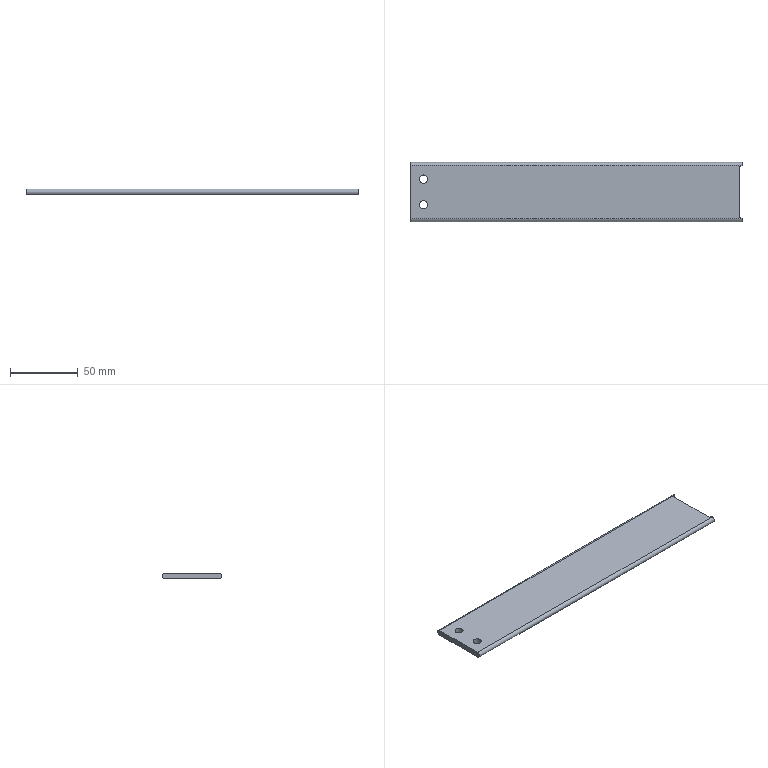Part | STEP file | Tube feed_id910_x_t | 1 solid | 12 faces | box 244.5 x 43.6 x 4.2 mm | volume 43290 mm3 | plane 8 | cylinder 4 | commonest cylinder face diameters 4.2 x2 6 x2
STEP:
#1=CARTESIAN_POINT('',(0.,0.,0.));
#2=DIRECTION('',(0.,0.,1.));
#3=DIRECTION('',(1.,0.,0.));
#4=AXIS2_PLACEMENT_3D('',#1,#2,#3);
#5=CARTESIAN_POINT('',(-309.5,-9.325,-1.3));
#6=VERTEX_POINT('',#5);
#7=CARTESIAN_POINT('',(-309.5,-9.664,-1.3));
#8=VERTEX_POINT('',#7);
#9=CARTESIAN_POINT('',(-309.5,29.736,-1.3));
#10=DIRECTION('',(0.,-1.,0.));
#11=VECTOR('',#10,1.);
#12=LINE('',#9,#11);
#13=CARTESIAN_POINT('',(-554.,29.736,-1.3));
#14=DIRECTION('',(0.,0.,1.));
#15=DIRECTION('',(0.,-1.,0.));
#16=AXIS2_PLACEMENT_3D('',#13,#14,#15);
#17=PLANE('',#16);
#18=CARTESIAN_POINT('',(0.,244.5));
#19=DIRECTION('',(1.,0.));
#20=VECTOR('',#19,1.);
#21=LINE('',#18,#20);
#22=(GEOMETRIC_REPRESENTATION_CONTEXT(2)PARAMETRIC_REPRESENTATION_CONTEXT()REPRESENTATION_CONTEXT('',''));
#23=DEFINITIONAL_REPRESENTATION('',(#21),#22);
#24=PCURVE('',#17,#23);
#25=CARTESIAN_POINT('',(-309.5,29.736,-3.15));
#26=DIRECTION('',(1.,0.,0.));
#27=DIRECTION('',(0.,0.,-1.));
#28=AXIS2_PLACEMENT_3D('',#25,#26,#27);
#29=PLANE('',#28);
#30=CARTESIAN_POINT('',(-1.85,0.));
#31=DIRECTION('',(0.,-1.));
#32=VECTOR('',#31,1.);
#33=LINE('',#30,#32);
#34=(GEOMETRIC_REPRESENTATION_CONTEXT(2)PARAMETRIC_REPRESENTATION_CONTEXT()REPRESENTATION_CONTEXT('',''));
#35=DEFINITIONAL_REPRESENTATION('',(#33),#34);
#36=PCURVE('',#29,#35);
#37=SURFACE_CURVE('',#12,(#24,#36),.PCURVE_S1.);
#38=EDGE_CURVE('',#6,#8,#37,.T.);
#39=ORIENTED_EDGE('',*,*,#38,.F.);
#40=CARTESIAN_POINT('',(-311.5,-8.629,-1.3));
#41=VERTEX_POINT('',#40);
#42=CARTESIAN_POINT('',(-539.725,70.769,-1.3));
#43=DIRECTION('',(-0.9445,0.3286,0.));
#44=VECTOR('',#43,1.);
#45=LINE('',#42,#44);
#46=CARTESIAN_POINT('',(-41.033,14.275));
#47=DIRECTION('',(-0.3286,-0.9445));
#48=VECTOR('',#47,1.);
#49=LINE('',#46,#48);
#50=(GEOMETRIC_REPRESENTATION_CONTEXT(2)PARAMETRIC_REPRESENTATION_CONTEXT()REPRESENTATION_CONTEXT('',''));
#51=DEFINITIONAL_REPRESENTATION('',(#49),#50);
#52=PCURVE('',#17,#51);
#53=CARTESIAN_POINT('',(-311.5,-8.629,48.7));
#54=DIRECTION('',(0.3286,0.9445,0.));
#55=DIRECTION('',(-0.9445,0.3286,0.));
#56=AXIS2_PLACEMENT_3D('',#53,#54,#55);
#57=PLANE('',#56);
#58=CARTESIAN_POINT('',(241.642,-50.));
#59=DIRECTION('',(1.,0.));
#60=VECTOR('',#59,1.);
#61=LINE('',#58,#60);
#62=(GEOMETRIC_REPRESENTATION_CONTEXT(2)PARAMETRIC_REPRESENTATION_CONTEXT()REPRESENTATION_CONTEXT('',''));
#63=DEFINITIONAL_REPRESENTATION('',(#61),#62);
#64=PCURVE('',#57,#63);
#65=SURFACE_CURVE('',#45,(#52,#64),.PCURVE_S1.);
#66=EDGE_CURVE('',#6,#41,#65,.T.);
#67=ORIENTED_EDGE('',*,*,#66,.T.);
#68=CARTESIAN_POINT('',(-311.5,28.701,-1.3));
#69=VERTEX_POINT('',#68);
#70=CARTESIAN_POINT('',(-311.5,29.736,-1.3));
#71=DIRECTION('',(0.,1.,0.));
#72=VECTOR('',#71,1.);
#73=LINE('',#70,#72);
#74=CARTESIAN_POINT('',(0.,242.5));
#75=DIRECTION('',(-1.,0.));
#76=VECTOR('',#75,1.);
#77=LINE('',#74,#76);
#78=(GEOMETRIC_REPRESENTATION_CONTEXT(2)PARAMETRIC_REPRESENTATION_CONTEXT()REPRESENTATION_CONTEXT('',''));
#79=DEFINITIONAL_REPRESENTATION('',(#77),#78);
#80=PCURVE('',#17,#79);
#81=CARTESIAN_POINT('',(-311.5,28.701,48.7));
#82=DIRECTION('',(1.,0.,0.));
#83=DIRECTION('',(0.,0.,-1.));
#84=AXIS2_PLACEMENT_3D('',#81,#82,#83);
#85=PLANE('',#84);
#86=CARTESIAN_POINT('',(50.,1.035));
#87=DIRECTION('',(0.,1.));
#88=VECTOR('',#87,1.);
#89=LINE('',#86,#88);
#90=(GEOMETRIC_REPRESENTATION_CONTEXT(2)PARAMETRIC_REPRESENTATION_CONTEXT()REPRESENTATION_CONTEXT('',''));
#91=DEFINITIONAL_REPRESENTATION('',(#89),#90);
#92=PCURVE('',#85,#91);
#93=SURFACE_CURVE('',#73,(#80,#92),.PCURVE_S1.);
#94=EDGE_CURVE('',#41,#69,#93,.T.);
#95=ORIENTED_EDGE('',*,*,#94,.T.);
#96=CARTESIAN_POINT('',(-309.5,29.396,-1.3));
#97=VERTEX_POINT('',#96);
#98=CARTESIAN_POINT('',(-527.498,-46.444,-1.3));
#99=DIRECTION('',(0.9445,0.3286,0.));
#100=VECTOR('',#99,1.);
#101=LINE('',#98,#100);
#102=CARTESIAN_POINT('',(76.179,26.502));
#103=DIRECTION('',(-0.3286,0.9445));
#104=VECTOR('',#103,1.);
#105=LINE('',#102,#104);
#106=(GEOMETRIC_REPRESENTATION_CONTEXT(2)PARAMETRIC_REPRESENTATION_CONTEXT()REPRESENTATION_CONTEXT('',''));
#107=DEFINITIONAL_REPRESENTATION('',(#105),#106);
#108=PCURVE('',#17,#107);
#109=CARTESIAN_POINT('',(-302.,32.005,48.7));
#110=DIRECTION('',(0.3286,-0.9445,0.));
#111=DIRECTION('',(0.9445,0.3286,0.));
#112=AXIS2_PLACEMENT_3D('',#109,#110,#111);
#113=PLANE('',#112);
#114=CARTESIAN_POINT('',(-238.754,-50.));
#115=DIRECTION('',(1.,0.));
#116=VECTOR('',#115,1.);
#117=LINE('',#114,#116);
#118=(GEOMETRIC_REPRESENTATION_CONTEXT(2)PARAMETRIC_REPRESENTATION_CONTEXT()REPRESENTATION_CONTEXT('',''));
#119=DEFINITIONAL_REPRESENTATION('',(#117),#118);
#120=PCURVE('',#113,#119);
#121=SURFACE_CURVE('',#101,(#108,#120),.PCURVE_S1.);
#122=EDGE_CURVE('',#69,#97,#121,.T.);
#123=ORIENTED_EDGE('',*,*,#122,.T.);
#124=CARTESIAN_POINT('',(-309.5,29.736,-1.3));
#125=VERTEX_POINT('',#124);
#126=CARTESIAN_POINT('',(-309.5,29.736,-1.3));
#127=DIRECTION('',(0.,-1.,0.));
#128=VECTOR('',#127,1.);
#129=LINE('',#126,#128);
#130=CARTESIAN_POINT('',(0.,244.5));
#131=DIRECTION('',(1.,0.));
#132=VECTOR('',#131,1.);
#133=LINE('',#130,#132);
#134=(GEOMETRIC_REPRESENTATION_CONTEXT(2)PARAMETRIC_REPRESENTATION_CONTEXT()REPRESENTATION_CONTEXT('',''));
#135=DEFINITIONAL_REPRESENTATION('',(#133),#134);
#136=PCURVE('',#17,#135);
#137=CARTESIAN_POINT('',(-309.5,29.736,-3.15));
#138=DIRECTION('',(1.,0.,0.));
#139=DIRECTION('',(0.,0.,-1.));
#140=AXIS2_PLACEMENT_3D('',#137,#138,#139);
#141=PLANE('',#140);
#142=CARTESIAN_POINT('',(-1.85,0.));
#143=DIRECTION('',(0.,-1.));
#144=VECTOR('',#143,1.);
#145=LINE('',#142,#144);
#146=(GEOMETRIC_REPRESENTATION_CONTEXT(2)PARAMETRIC_REPRESENTATION_CONTEXT()REPRESENTATION_CONTEXT('',''));
#147=DEFINITIONAL_REPRESENTATION('',(#145),#146);
#148=PCURVE('',#141,#147);
#149=SURFACE_CURVE('',#129,(#136,#148),.PCURVE_S1.);
#150=EDGE_CURVE('',#125,#97,#149,.T.);
#151=ORIENTED_EDGE('',*,*,#150,.F.);
#152=CARTESIAN_POINT('',(-554.,29.736,-1.3));
#153=VERTEX_POINT('',#152);
#154=CARTESIAN_POINT('',(-401.5,29.736,-1.3));
#155=DIRECTION('',(1.,0.,0.));
#156=VECTOR('',#155,1.);
#157=LINE('',#154,#156);
#158=CARTESIAN_POINT('',(0.,152.5));
#159=DIRECTION('',(0.,1.));
#160=VECTOR('',#159,1.);
#161=LINE('',#158,#160);
#162=(GEOMETRIC_REPRESENTATION_CONTEXT(2)PARAMETRIC_REPRESENTATION_CONTEXT()REPRESENTATION_CONTEXT('',''));
#163=DEFINITIONAL_REPRESENTATION('',(#161),#162);
#164=PCURVE('',#17,#163);
#165=CARTESIAN_POINT('',(-554.,29.736,-3.4));
#166=DIRECTION('',(1.,0.,0.));
#167=DIRECTION('',(0.,0.,-1.));
#168=AXIS2_PLACEMENT_3D('',#165,#166,#167);
#169=CYLINDRICAL_SURFACE('',#168,2.1);
#170=CARTESIAN_POINT('',(3.142,152.5));
#171=DIRECTION('',(0.,1.));
#172=VECTOR('',#171,1.);
#173=LINE('',#170,#172);
#174=(GEOMETRIC_REPRESENTATION_CONTEXT(2)PARAMETRIC_REPRESENTATION_CONTEXT()REPRESENTATION_CONTEXT('',''));
#175=DEFINITIONAL_REPRESENTATION('',(#173),#174);
#176=PCURVE('',#169,#175);
#177=SURFACE_CURVE('',#157,(#164,#176),.PCURVE_S1.);
#178=EDGE_CURVE('',#153,#125,#177,.T.);
#179=ORIENTED_EDGE('',*,*,#178,.F.);
#180=CARTESIAN_POINT('',(-554.,-9.664,-1.3));
#181=VERTEX_POINT('',#180);
#182=CARTESIAN_POINT('',(-554.,29.736,-1.3));
#183=DIRECTION('',(0.,-1.,0.));
#184=VECTOR('',#183,1.);
#185=LINE('',#182,#184);
#186=CARTESIAN_POINT('',(0.,0.));
#187=DIRECTION('',(1.,0.));
#188=VECTOR('',#187,1.);
#189=LINE('',#186,#188);
#190=(GEOMETRIC_REPRESENTATION_CONTEXT(2)PARAMETRIC_REPRESENTATION_CONTEXT()REPRESENTATION_CONTEXT('',''));
#191=DEFINITIONAL_REPRESENTATION('',(#189),#190);
#192=PCURVE('',#17,#191);
#193=CARTESIAN_POINT('',(-554.,29.736,-3.15));
#194=DIRECTION('',(1.,0.,0.));
#195=DIRECTION('',(0.,0.,-1.));
#196=AXIS2_PLACEMENT_3D('',#193,#194,#195);
#197=PLANE('',#196);
#198=CARTESIAN_POINT('',(-1.85,0.));
#199=DIRECTION('',(0.,-1.));
#200=VECTOR('',#199,1.);
#201=LINE('',#198,#200);
#202=(GEOMETRIC_REPRESENTATION_CONTEXT(2)PARAMETRIC_REPRESENTATION_CONTEXT()REPRESENTATION_CONTEXT('',''));
#203=DEFINITIONAL_REPRESENTATION('',(#201),#202);
#204=PCURVE('',#197,#203);
#205=SURFACE_CURVE('',#185,(#192,#204),.PCURVE_S1.);
#206=EDGE_CURVE('',#153,#181,#205,.T.);
#207=ORIENTED_EDGE('',*,*,#206,.T.);
#208=CARTESIAN_POINT('',(-401.5,-9.664,-1.3));
#209=DIRECTION('',(1.,0.,0.));
#210=VECTOR('',#209,1.);
#211=LINE('',#208,#210);
#212=CARTESIAN_POINT('',(39.4,152.5));
#213=DIRECTION('',(0.,1.));
#214=VECTOR('',#213,1.);
#215=LINE('',#212,#214);
#216=(GEOMETRIC_REPRESENTATION_CONTEXT(2)PARAMETRIC_REPRESENTATION_CONTEXT()REPRESENTATION_CONTEXT('',''));
#217=DEFINITIONAL_REPRESENTATION('',(#215),#216);
#218=PCURVE('',#17,#217);
#219=CARTESIAN_POINT('',(-554.,-9.664,-3.4));
#220=DIRECTION('',(1.,0.,0.));
#221=DIRECTION('',(0.,0.,-1.));
#222=AXIS2_PLACEMENT_3D('',#219,#220,#221);
#223=CYLINDRICAL_SURFACE('',#222,2.1);
#224=CARTESIAN_POINT('',(3.142,152.5));
#225=DIRECTION('',(0.,1.));
#226=VECTOR('',#225,1.);
#227=LINE('',#224,#226);
#228=(GEOMETRIC_REPRESENTATION_CONTEXT(2)PARAMETRIC_REPRESENTATION_CONTEXT()REPRESENTATION_CONTEXT('',''));
#229=DEFINITIONAL_REPRESENTATION('',(#227),#228);
#230=PCURVE('',#223,#229);
#231=SURFACE_CURVE('',#211,(#218,#230),.PCURVE_S1.);
#232=EDGE_CURVE('',#181,#8,#231,.T.);
#233=ORIENTED_EDGE('',*,*,#232,.T.);
#234=EDGE_LOOP('',(#39,#67,#95,#123,#151,#179,#207,#233));
#235=FACE_BOUND('',#234,.T.);
#236=CARTESIAN_POINT('',(-544.,16.556,-1.3));
#237=VERTEX_POINT('',#236);
#238=CARTESIAN_POINT('',(-544.,22.556,-1.3));
#239=VERTEX_POINT('',#238);
#240=CARTESIAN_POINT('',(-544.,19.556,-1.3));
#241=DIRECTION('',(0.,0.,1.));
#242=DIRECTION('',(0.,-1.,0.));
#243=AXIS2_PLACEMENT_3D('',#240,#241,#242);
#244=CIRCLE('',#243,3.);
#245=CARTESIAN_POINT('',(10.18,10.));
#246=DIRECTION('',(1.,0.));
#247=AXIS2_PLACEMENT_2D('',#245,#246);
#248=CIRCLE('',#247,3.);
#249=(GEOMETRIC_REPRESENTATION_CONTEXT(2)PARAMETRIC_REPRESENTATION_CONTEXT()REPRESENTATION_CONTEXT('',''));
#250=DEFINITIONAL_REPRESENTATION('',(#248),#249);
#251=PCURVE('',#17,#250);
#252=CARTESIAN_POINT('',(-544.,19.556,-40.9));
#253=DIRECTION('',(0.,0.,1.));
#254=DIRECTION('',(1.,0.,0.));
#255=AXIS2_PLACEMENT_3D('',#252,#253,#254);
#256=CYLINDRICAL_SURFACE('',#255,3.);
#257=CARTESIAN_POINT('',(4.712,39.6));
#258=DIRECTION('',(1.,0.));
#259=VECTOR('',#258,1.);
#260=LINE('',#257,#259);
#261=(GEOMETRIC_REPRESENTATION_CONTEXT(2)PARAMETRIC_REPRESENTATION_CONTEXT()REPRESENTATION_CONTEXT('',''));
#262=DEFINITIONAL_REPRESENTATION('',(#260),#261);
#263=PCURVE('',#256,#262);
#264=SURFACE_CURVE('',#244,(#251,#263),.PCURVE_S1.);
#265=EDGE_CURVE('',#237,#239,#264,.T.);
#266=ORIENTED_EDGE('',*,*,#265,.F.);
#267=CARTESIAN_POINT('',(-544.,19.556,-1.3));
#268=DIRECTION('',(0.,0.,1.));
#269=DIRECTION('',(0.,-1.,0.));
#270=AXIS2_PLACEMENT_3D('',#267,#268,#269);
#271=CIRCLE('',#270,3.);
#272=CARTESIAN_POINT('',(10.18,10.));
#273=DIRECTION('',(1.,0.));
#274=AXIS2_PLACEMENT_2D('',#272,#273);
#275=CIRCLE('',#274,3.);
#276=(GEOMETRIC_REPRESENTATION_CONTEXT(2)PARAMETRIC_REPRESENTATION_CONTEXT()REPRESENTATION_CONTEXT('',''));
#277=DEFINITIONAL_REPRESENTATION('',(#275),#276);
#278=PCURVE('',#17,#277);
#279=CARTESIAN_POINT('',(-1.571,39.6));
#280=DIRECTION('',(1.,0.));
#281=VECTOR('',#280,1.);
#282=LINE('',#279,#281);
#283=(GEOMETRIC_REPRESENTATION_CONTEXT(2)PARAMETRIC_REPRESENTATION_CONTEXT()REPRESENTATION_CONTEXT('',''));
#284=DEFINITIONAL_REPRESENTATION('',(#282),#283);
#285=PCURVE('',#256,#284);
#286=SURFACE_CURVE('',#271,(#278,#285),.PCURVE_S1.);
#287=EDGE_CURVE('',#239,#237,#286,.T.);
#288=ORIENTED_EDGE('',*,*,#287,.F.);
#289=EDGE_LOOP('',(#266,#288));
#290=FACE_BOUND('',#289,.T.);
#291=CARTESIAN_POINT('',(-544.,-2.444,-1.3));
#292=VERTEX_POINT('',#291);
#293=CARTESIAN_POINT('',(-544.,3.556,-1.3));
#294=VERTEX_POINT('',#293);
#295=CARTESIAN_POINT('',(-544.,0.5556,-1.3));
#296=DIRECTION('',(0.,0.,-1.));
#297=DIRECTION('',(0.,-1.,0.));
#298=AXIS2_PLACEMENT_3D('',#295,#296,#297);
#299=CIRCLE('',#298,3.);
#300=CARTESIAN_POINT('',(32.18,10.));
#301=CARTESIAN_POINT('',(32.18,4.804));
#302=CARTESIAN_POINT('',(27.68,7.402));
#303=CARTESIAN_POINT('',(23.18,10.));
#304=CARTESIAN_POINT('',(27.68,12.598));
#305=CARTESIAN_POINT('',(32.18,15.196));
#306=CARTESIAN_POINT('',(32.18,10.));
#307=(BOUNDED_CURVE()B_SPLINE_CURVE(2,(#300,#301,#302,#303,#304,#305,#306),.UNSPECIFIED.,.T.,.F.)B_SPLINE_CURVE_WITH_KNOTS((1,2,2,2,2,1),(-2.094,0.,2.094,4.189,6.283,8.378),.UNSPECIFIED.)CURVE()GEOMETRIC_REPRESENTATION_ITEM()RATIONAL_B_SPLINE_CURVE((1.,0.5,1.,0.5,1.,0.5,1.))REPRESENTATION_ITEM(''));
#308=(GEOMETRIC_REPRESENTATION_CONTEXT(2)PARAMETRIC_REPRESENTATION_CONTEXT()REPRESENTATION_CONTEXT('',''));
#309=DEFINITIONAL_REPRESENTATION('',(#307),#308);
#310=PCURVE('',#17,#309);
#311=CARTESIAN_POINT('',(-544.,0.5556,-40.9));
#312=DIRECTION('',(0.,0.,1.));
#313=DIRECTION('',(1.,0.,0.));
#314=AXIS2_PLACEMENT_3D('',#311,#312,#313);
#315=CYLINDRICAL_SURFACE('',#314,3.);
#316=CARTESIAN_POINT('',(4.712,39.6));
#317=DIRECTION('',(-1.,0.));
#318=VECTOR('',#317,1.);
#319=LINE('',#316,#318);
#320=(GEOMETRIC_REPRESENTATION_CONTEXT(2)PARAMETRIC_REPRESENTATION_CONTEXT()REPRESENTATION_CONTEXT('',''));
#321=DEFINITIONAL_REPRESENTATION('',(#319),#320);
#322=PCURVE('',#315,#321);
#323=SURFACE_CURVE('',#299,(#310,#322),.PCURVE_S1.);
#324=EDGE_CURVE('',#292,#294,#323,.T.);
#325=ORIENTED_EDGE('',*,*,#324,.T.);
#326=CARTESIAN_POINT('',(-544.,0.5556,-1.3));
#327=DIRECTION('',(0.,0.,-1.));
#328=DIRECTION('',(0.,-1.,0.));
#329=AXIS2_PLACEMENT_3D('',#326,#327,#328);
#330=CIRCLE('',#329,3.);
#331=CARTESIAN_POINT('',(32.18,10.));
#332=CARTESIAN_POINT('',(32.18,4.804));
#333=CARTESIAN_POINT('',(27.68,7.402));
#334=CARTESIAN_POINT('',(23.18,10.));
#335=CARTESIAN_POINT('',(27.68,12.598));
#336=CARTESIAN_POINT('',(32.18,15.196));
#337=CARTESIAN_POINT('',(32.18,10.));
#338=(BOUNDED_CURVE()B_SPLINE_CURVE(2,(#331,#332,#333,#334,#335,#336,#337),.UNSPECIFIED.,.T.,.F.)B_SPLINE_CURVE_WITH_KNOTS((1,2,2,2,2,1),(-2.094,0.,2.094,4.189,6.283,8.378),.UNSPECIFIED.)CURVE()GEOMETRIC_REPRESENTATION_ITEM()RATIONAL_B_SPLINE_CURVE((1.,0.5,1.,0.5,1.,0.5,1.))REPRESENTATION_ITEM(''));
#339=(GEOMETRIC_REPRESENTATION_CONTEXT(2)PARAMETRIC_REPRESENTATION_CONTEXT()REPRESENTATION_CONTEXT('',''));
#340=DEFINITIONAL_REPRESENTATION('',(#338),#339);
#341=PCURVE('',#17,#340);
#342=CARTESIAN_POINT('',(10.996,39.6));
#343=DIRECTION('',(-1.,0.));
#344=VECTOR('',#343,1.);
#345=LINE('',#342,#344);
#346=(GEOMETRIC_REPRESENTATION_CONTEXT(2)PARAMETRIC_REPRESENTATION_CONTEXT()REPRESENTATION_CONTEXT('',''));
#347=DEFINITIONAL_REPRESENTATION('',(#345),#346);
#348=PCURVE('',#315,#347);
#349=SURFACE_CURVE('',#330,(#341,#348),.PCURVE_S1.);
#350=EDGE_CURVE('',#294,#292,#349,.T.);
#351=ORIENTED_EDGE('',*,*,#350,.T.);
#352=EDGE_LOOP('',(#325,#351));
#353=FACE_BOUND('',#352,.T.);
#354=ADVANCED_FACE('',(#235,#290,#353),#17,.T.);
#355=CARTESIAN_POINT('',(-311.5,28.701,-5.5));
#356=VERTEX_POINT('',#355);
#357=CARTESIAN_POINT('',(-311.5,-8.629,-5.5));
#358=VERTEX_POINT('',#357);
#359=CARTESIAN_POINT('',(-311.5,-9.664,-5.5));
#360=DIRECTION('',(0.,-1.,0.));
#361=VECTOR('',#360,1.);
#362=LINE('',#359,#361);
#363=CARTESIAN_POINT('',(-554.,-9.664,-5.5));
#364=DIRECTION('',(0.,0.,-1.));
#365=DIRECTION('',(0.,1.,0.));
#366=AXIS2_PLACEMENT_3D('',#363,#364,#365);
#367=PLANE('',#366);
#368=CARTESIAN_POINT('',(0.,242.5));
#369=DIRECTION('',(-1.,0.));
#370=VECTOR('',#369,1.);
#371=LINE('',#368,#370);
#372=(GEOMETRIC_REPRESENTATION_CONTEXT(2)PARAMETRIC_REPRESENTATION_CONTEXT()REPRESENTATION_CONTEXT('',''));
#373=DEFINITIONAL_REPRESENTATION('',(#371),#372);
#374=PCURVE('',#367,#373);
#375=CARTESIAN_POINT('',(54.2,-38.365));
#376=DIRECTION('',(0.,-1.));
#377=VECTOR('',#376,1.);
#378=LINE('',#375,#377);
#379=(GEOMETRIC_REPRESENTATION_CONTEXT(2)PARAMETRIC_REPRESENTATION_CONTEXT()REPRESENTATION_CONTEXT('',''));
#380=DEFINITIONAL_REPRESENTATION('',(#378),#379);
#381=PCURVE('',#85,#380);
#382=SURFACE_CURVE('',#362,(#374,#381),.PCURVE_S1.);
#383=EDGE_CURVE('',#356,#358,#382,.T.);
#384=ORIENTED_EDGE('',*,*,#383,.T.);
#385=CARTESIAN_POINT('',(-309.5,-9.325,-5.5));
#386=VERTEX_POINT('',#385);
#387=CARTESIAN_POINT('',(-527.498,66.515,-5.5));
#388=DIRECTION('',(0.9445,-0.3286,0.));
#389=VECTOR('',#388,1.);
#390=LINE('',#387,#389);
#391=CARTESIAN_POINT('',(76.179,26.502));
#392=DIRECTION('',(-0.3286,0.9445));
#393=VECTOR('',#392,1.);
#394=LINE('',#391,#393);
#395=(GEOMETRIC_REPRESENTATION_CONTEXT(2)PARAMETRIC_REPRESENTATION_CONTEXT()REPRESENTATION_CONTEXT('',''));
#396=DEFINITIONAL_REPRESENTATION('',(#394),#395);
#397=PCURVE('',#367,#396);
#398=CARTESIAN_POINT('',(228.696,-54.2));
#399=DIRECTION('',(-1.,0.));
#400=VECTOR('',#399,1.);
#401=LINE('',#398,#400);
#402=(GEOMETRIC_REPRESENTATION_CONTEXT(2)PARAMETRIC_REPRESENTATION_CONTEXT()REPRESENTATION_CONTEXT('',''));
#403=DEFINITIONAL_REPRESENTATION('',(#401),#402);
#404=PCURVE('',#57,#403);
#405=SURFACE_CURVE('',#390,(#397,#404),.PCURVE_S1.);
#406=EDGE_CURVE('',#358,#386,#405,.T.);
#407=ORIENTED_EDGE('',*,*,#406,.T.);
#408=CARTESIAN_POINT('',(-309.5,-9.664,-5.5));
#409=VERTEX_POINT('',#408);
#410=CARTESIAN_POINT('',(-309.5,29.736,-5.5));
#411=DIRECTION('',(0.,1.,0.));
#412=VECTOR('',#411,1.);
#413=LINE('',#410,#412);
#414=CARTESIAN_POINT('',(39.4,244.5));
#415=DIRECTION('',(1.,0.));
#416=VECTOR('',#415,1.);
#417=LINE('',#414,#416);
#418=(GEOMETRIC_REPRESENTATION_CONTEXT(2)PARAMETRIC_REPRESENTATION_CONTEXT()REPRESENTATION_CONTEXT('',''));
#419=DEFINITIONAL_REPRESENTATION('',(#417),#418);
#420=PCURVE('',#367,#419);
#421=CARTESIAN_POINT('',(2.35,0.));
#422=DIRECTION('',(0.,1.));
#423=VECTOR('',#422,1.);
#424=LINE('',#421,#423);
#425=(GEOMETRIC_REPRESENTATION_CONTEXT(2)PARAMETRIC_REPRESENTATION_CONTEXT()REPRESENTATION_CONTEXT('',''));
#426=DEFINITIONAL_REPRESENTATION('',(#424),#425);
#427=PCURVE('',#29,#426);
#428=SURFACE_CURVE('',#413,(#420,#427),.PCURVE_S1.);
#429=EDGE_CURVE('',#409,#386,#428,.T.);
#430=ORIENTED_EDGE('',*,*,#429,.F.);
#431=CARTESIAN_POINT('',(-554.,-9.664,-5.5));
#432=VERTEX_POINT('',#431);
#433=CARTESIAN_POINT('',(-401.5,-9.664,-5.5));
#434=DIRECTION('',(1.,0.,0.));
#435=VECTOR('',#434,1.);
#436=LINE('',#433,#435);
#437=CARTESIAN_POINT('',(0.,152.5));
#438=DIRECTION('',(0.,1.));
#439=VECTOR('',#438,1.);
#440=LINE('',#437,#439);
#441=(GEOMETRIC_REPRESENTATION_CONTEXT(2)PARAMETRIC_REPRESENTATION_CONTEXT()REPRESENTATION_CONTEXT('',''));
#442=DEFINITIONAL_REPRESENTATION('',(#440),#441);
#443=PCURVE('',#367,#442);
#444=CARTESIAN_POINT('',(6.283,152.5));
#445=DIRECTION('',(0.,1.));
#446=VECTOR('',#445,1.);
#447=LINE('',#444,#446);
#448=(GEOMETRIC_REPRESENTATION_CONTEXT(2)PARAMETRIC_REPRESENTATION_CONTEXT()REPRESENTATION_CONTEXT('',''));
#449=DEFINITIONAL_REPRESENTATION('',(#447),#448);
#450=PCURVE('',#223,#449);
#451=SURFACE_CURVE('',#436,(#443,#450),.PCURVE_S1.);
#452=EDGE_CURVE('',#432,#409,#451,.T.);
#453=ORIENTED_EDGE('',*,*,#452,.F.);
#454=CARTESIAN_POINT('',(-554.,29.736,-5.5));
#455=VERTEX_POINT('',#454);
#456=CARTESIAN_POINT('',(-554.,-9.664,-5.5));
#457=DIRECTION('',(0.,1.,0.));
#458=VECTOR('',#457,1.);
#459=LINE('',#456,#458);
#460=CARTESIAN_POINT('',(0.,0.));
#461=DIRECTION('',(1.,0.));
#462=VECTOR('',#461,1.);
#463=LINE('',#460,#462);
#464=(GEOMETRIC_REPRESENTATION_CONTEXT(2)PARAMETRIC_REPRESENTATION_CONTEXT()REPRESENTATION_CONTEXT('',''));
#465=DEFINITIONAL_REPRESENTATION('',(#463),#464);
#466=PCURVE('',#367,#465);
#467=CARTESIAN_POINT('',(2.35,-39.4));
#468=DIRECTION('',(0.,1.));
#469=VECTOR('',#468,1.);
#470=LINE('',#467,#469);
#471=(GEOMETRIC_REPRESENTATION_CONTEXT(2)PARAMETRIC_REPRESENTATION_CONTEXT()REPRESENTATION_CONTEXT('',''));
#472=DEFINITIONAL_REPRESENTATION('',(#470),#471);
#473=PCURVE('',#197,#472);
#474=SURFACE_CURVE('',#459,(#466,#473),.PCURVE_S1.);
#475=EDGE_CURVE('',#432,#455,#474,.T.);
#476=ORIENTED_EDGE('',*,*,#475,.T.);
#477=CARTESIAN_POINT('',(-309.5,29.736,-5.5));
#478=VERTEX_POINT('',#477);
#479=CARTESIAN_POINT('',(-401.5,29.736,-5.5));
#480=DIRECTION('',(1.,0.,0.));
#481=VECTOR('',#480,1.);
#482=LINE('',#479,#481);
#483=CARTESIAN_POINT('',(39.4,152.5));
#484=DIRECTION('',(0.,1.));
#485=VECTOR('',#484,1.);
#486=LINE('',#483,#485);
#487=(GEOMETRIC_REPRESENTATION_CONTEXT(2)PARAMETRIC_REPRESENTATION_CONTEXT()REPRESENTATION_CONTEXT('',''));
#488=DEFINITIONAL_REPRESENTATION('',(#486),#487);
#489=PCURVE('',#367,#488);
#490=CARTESIAN_POINT('',(0.,152.5));
#491=DIRECTION('',(0.,1.));
#492=VECTOR('',#491,1.);
#493=LINE('',#490,#492);
#494=(GEOMETRIC_REPRESENTATION_CONTEXT(2)PARAMETRIC_REPRESENTATION_CONTEXT()REPRESENTATION_CONTEXT('',''));
#495=DEFINITIONAL_REPRESENTATION('',(#493),#494);
#496=PCURVE('',#169,#495);
#497=SURFACE_CURVE('',#482,(#489,#496),.PCURVE_S1.);
#498=EDGE_CURVE('',#455,#478,#497,.T.);
#499=ORIENTED_EDGE('',*,*,#498,.T.);
#500=CARTESIAN_POINT('',(-309.5,29.396,-5.5));
#501=VERTEX_POINT('',#500);
#502=CARTESIAN_POINT('',(-309.5,29.736,-5.5));
#503=DIRECTION('',(0.,1.,0.));
#504=VECTOR('',#503,1.);
#505=LINE('',#502,#504);
#506=CARTESIAN_POINT('',(39.4,244.5));
#507=DIRECTION('',(1.,0.));
#508=VECTOR('',#507,1.);
#509=LINE('',#506,#508);
#510=(GEOMETRIC_REPRESENTATION_CONTEXT(2)PARAMETRIC_REPRESENTATION_CONTEXT()REPRESENTATION_CONTEXT('',''));
#511=DEFINITIONAL_REPRESENTATION('',(#509),#510);
#512=PCURVE('',#367,#511);
#513=CARTESIAN_POINT('',(2.35,0.));
#514=DIRECTION('',(0.,1.));
#515=VECTOR('',#514,1.);
#516=LINE('',#513,#515);
#517=(GEOMETRIC_REPRESENTATION_CONTEXT(2)PARAMETRIC_REPRESENTATION_CONTEXT()REPRESENTATION_CONTEXT('',''));
#518=DEFINITIONAL_REPRESENTATION('',(#516),#517);
#519=PCURVE('',#141,#518);
#520=SURFACE_CURVE('',#505,(#512,#519),.PCURVE_S1.);
#521=EDGE_CURVE('',#501,#478,#520,.T.);
#522=ORIENTED_EDGE('',*,*,#521,.F.);
#523=CARTESIAN_POINT('',(-539.725,-50.697,-5.5));
#524=DIRECTION('',(-0.9445,-0.3286,0.));
#525=VECTOR('',#524,1.);
#526=LINE('',#523,#525);
#527=CARTESIAN_POINT('',(-41.033,14.275));
#528=DIRECTION('',(-0.3286,-0.9445));
#529=VECTOR('',#528,1.);
#530=LINE('',#527,#529);
#531=(GEOMETRIC_REPRESENTATION_CONTEXT(2)PARAMETRIC_REPRESENTATION_CONTEXT()REPRESENTATION_CONTEXT('',''));
#532=DEFINITIONAL_REPRESENTATION('',(#530),#531);
#533=PCURVE('',#367,#532);
#534=CARTESIAN_POINT('',(-251.7,-54.2));
#535=DIRECTION('',(-1.,0.));
#536=VECTOR('',#535,1.);
#537=LINE('',#534,#536);
#538=(GEOMETRIC_REPRESENTATION_CONTEXT(2)PARAMETRIC_REPRESENTATION_CONTEXT()REPRESENTATION_CONTEXT('',''));
#539=DEFINITIONAL_REPRESENTATION('',(#537),#538);
#540=PCURVE('',#113,#539);
#541=SURFACE_CURVE('',#526,(#533,#540),.PCURVE_S1.);
#542=EDGE_CURVE('',#501,#356,#541,.T.);
#543=ORIENTED_EDGE('',*,*,#542,.T.);
#544=EDGE_LOOP('',(#384,#407,#430,#453,#476,#499,#522,#543));
#545=FACE_BOUND('',#544,.T.);
#546=CARTESIAN_POINT('',(-544.,22.556,-5.5));
#547=VERTEX_POINT('',#546);
#548=CARTESIAN_POINT('',(-544.,19.556,-5.5));
#549=DIRECTION('',(0.,0.,-1.));
#550=DIRECTION('',(0.,1.,0.));
#551=AXIS2_PLACEMENT_3D('',#548,#549,#550);
#552=CIRCLE('',#551,3.);
#553=CARTESIAN_POINT('',(29.22,10.));
#554=DIRECTION('',(1.,0.));
#555=AXIS2_PLACEMENT_2D('',#553,#554);
#556=CIRCLE('',#555,3.);
#557=(GEOMETRIC_REPRESENTATION_CONTEXT(2)PARAMETRIC_REPRESENTATION_CONTEXT()REPRESENTATION_CONTEXT('',''));
#558=DEFINITIONAL_REPRESENTATION('',(#556),#557);
#559=PCURVE('',#367,#558);
#560=CARTESIAN_POINT('',(7.854,35.4));
#561=DIRECTION('',(-1.,0.));
#562=VECTOR('',#561,1.);
#563=LINE('',#560,#562);
#564=(GEOMETRIC_REPRESENTATION_CONTEXT(2)PARAMETRIC_REPRESENTATION_CONTEXT()REPRESENTATION_CONTEXT('',''));
#565=DEFINITIONAL_REPRESENTATION('',(#563),#564);
#566=PCURVE('',#256,#565);
#567=SURFACE_CURVE('',#552,(#559,#566),.PCURVE_S1.);
#568=EDGE_CURVE('',#547,#547,#567,.T.);
#569=ORIENTED_EDGE('',*,*,#568,.F.);
#570=EDGE_LOOP('',(#569));
#571=FACE_BOUND('',#570,.T.);
#572=CARTESIAN_POINT('',(-544.,3.556,-5.5));
#573=VERTEX_POINT('',#572);
#574=CARTESIAN_POINT('',(-544.,0.5556,-5.5));
#575=DIRECTION('',(0.,0.,1.));
#576=DIRECTION('',(0.,1.,0.));
#577=AXIS2_PLACEMENT_3D('',#574,#575,#576);
#578=CIRCLE('',#577,3.);
#579=CARTESIAN_POINT('',(13.22,10.));
#580=CARTESIAN_POINT('',(13.22,4.804));
#581=CARTESIAN_POINT('',(8.72,7.402));
#582=CARTESIAN_POINT('',(4.22,10.));
#583=CARTESIAN_POINT('',(8.72,12.598));
#584=CARTESIAN_POINT('',(13.22,15.196));
#585=CARTESIAN_POINT('',(13.22,10.));
#586=(BOUNDED_CURVE()B_SPLINE_CURVE(2,(#579,#580,#581,#582,#583,#584,#585),.UNSPECIFIED.,.T.,.F.)B_SPLINE_CURVE_WITH_KNOTS((1,2,2,2,2,1),(-2.094,0.,2.094,4.189,6.283,8.378),.UNSPECIFIED.)CURVE()GEOMETRIC_REPRESENTATION_ITEM()RATIONAL_B_SPLINE_CURVE((1.,0.5,1.,0.5,1.,0.5,1.))REPRESENTATION_ITEM(''));
#587=(GEOMETRIC_REPRESENTATION_CONTEXT(2)PARAMETRIC_REPRESENTATION_CONTEXT()REPRESENTATION_CONTEXT('',''));
#588=DEFINITIONAL_REPRESENTATION('',(#586),#587);
#589=PCURVE('',#367,#588);
#590=CARTESIAN_POINT('',(1.571,35.4));
#591=DIRECTION('',(1.,0.));
#592=VECTOR('',#591,1.);
#593=LINE('',#590,#592);
#594=(GEOMETRIC_REPRESENTATION_CONTEXT(2)PARAMETRIC_REPRESENTATION_CONTEXT()REPRESENTATION_CONTEXT('',''));
#595=DEFINITIONAL_REPRESENTATION('',(#593),#594);
#596=PCURVE('',#315,#595);
#597=SURFACE_CURVE('',#578,(#589,#596),.PCURVE_S1.);
#598=EDGE_CURVE('',#573,#573,#597,.T.);
#599=ORIENTED_EDGE('',*,*,#598,.T.);
#600=EDGE_LOOP('',(#599));
#601=FACE_BOUND('',#600,.T.);
#602=ADVANCED_FACE('',(#545,#571,#601),#367,.T.);
#603=ORIENTED_EDGE('',*,*,#429,.T.);
#604=CARTESIAN_POINT('',(-309.5,-9.325,-3.15));
#605=DIRECTION('',(0.,0.,1.));
#606=VECTOR('',#605,1.);
#607=LINE('',#604,#606);
#608=CARTESIAN_POINT('',(0.,-39.061));
#609=DIRECTION('',(-1.,0.));
#610=VECTOR('',#609,1.);
#611=LINE('',#608,#610);
#612=(GEOMETRIC_REPRESENTATION_CONTEXT(2)PARAMETRIC_REPRESENTATION_CONTEXT()REPRESENTATION_CONTEXT('',''));
#613=DEFINITIONAL_REPRESENTATION('',(#611),#612);
#614=PCURVE('',#29,#613);
#615=CARTESIAN_POINT('',(-2.118,-51.85));
#616=DIRECTION('',(0.,1.));
#617=VECTOR('',#616,1.);
#618=LINE('',#615,#617);
#619=(GEOMETRIC_REPRESENTATION_CONTEXT(2)PARAMETRIC_REPRESENTATION_CONTEXT()REPRESENTATION_CONTEXT('',''));
#620=DEFINITIONAL_REPRESENTATION('',(#618),#619);
#621=PCURVE('',#57,#620);
#622=SURFACE_CURVE('',#607,(#614,#621),.PCURVE_S1.);
#623=EDGE_CURVE('',#386,#6,#622,.T.);
#624=ORIENTED_EDGE('',*,*,#623,.T.);
#625=ORIENTED_EDGE('',*,*,#38,.T.);
#626=CARTESIAN_POINT('',(-309.5,-9.664,-3.4));
#627=DIRECTION('',(1.,0.,0.));
#628=DIRECTION('',(0.,0.,-1.));
#629=AXIS2_PLACEMENT_3D('',#626,#627,#628);
#630=CIRCLE('',#629,2.1);
#631=CARTESIAN_POINT('',(0.25,-39.4));
#632=DIRECTION('',(1.,0.));
#633=AXIS2_PLACEMENT_2D('',#631,#632);
#634=CIRCLE('',#633,2.1);
#635=(GEOMETRIC_REPRESENTATION_CONTEXT(2)PARAMETRIC_REPRESENTATION_CONTEXT()REPRESENTATION_CONTEXT('',''));
#636=DEFINITIONAL_REPRESENTATION('',(#634),#635);
#637=PCURVE('',#29,#636);
#638=CARTESIAN_POINT('',(0.,244.5));
#639=DIRECTION('',(1.,0.));
#640=VECTOR('',#639,1.);
#641=LINE('',#638,#640);
#642=(GEOMETRIC_REPRESENTATION_CONTEXT(2)PARAMETRIC_REPRESENTATION_CONTEXT()REPRESENTATION_CONTEXT('',''));
#643=DEFINITIONAL_REPRESENTATION('',(#641),#642);
#644=PCURVE('',#223,#643);
#645=SURFACE_CURVE('',#630,(#637,#644),.PCURVE_S1.);
#646=EDGE_CURVE('',#8,#409,#645,.T.);
#647=ORIENTED_EDGE('',*,*,#646,.T.);
#648=EDGE_LOOP('',(#603,#624,#625,#647));
#649=FACE_BOUND('',#648,.T.);
#650=ADVANCED_FACE('',(#649),#29,.T.);
#651=ORIENTED_EDGE('',*,*,#150,.T.);
#652=CARTESIAN_POINT('',(-309.5,29.396,-3.15));
#653=DIRECTION('',(0.,0.,-1.));
#654=VECTOR('',#653,1.);
#655=LINE('',#652,#654);
#656=CARTESIAN_POINT('',(0.,-0.3393));
#657=DIRECTION('',(1.,0.));
#658=VECTOR('',#657,1.);
#659=LINE('',#656,#658);
#660=(GEOMETRIC_REPRESENTATION_CONTEXT(2)PARAMETRIC_REPRESENTATION_CONTEXT()REPRESENTATION_CONTEXT('',''));
#661=DEFINITIONAL_REPRESENTATION('',(#659),#660);
#662=PCURVE('',#141,#661);
#663=CARTESIAN_POINT('',(-7.941,-51.85));
#664=DIRECTION('',(0.,-1.));
#665=VECTOR('',#664,1.);
#666=LINE('',#663,#665);
#667=(GEOMETRIC_REPRESENTATION_CONTEXT(2)PARAMETRIC_REPRESENTATION_CONTEXT()REPRESENTATION_CONTEXT('',''));
#668=DEFINITIONAL_REPRESENTATION('',(#666),#667);
#669=PCURVE('',#113,#668);
#670=SURFACE_CURVE('',#655,(#662,#669),.PCURVE_S1.);
#671=EDGE_CURVE('',#97,#501,#670,.T.);
#672=ORIENTED_EDGE('',*,*,#671,.T.);
#673=ORIENTED_EDGE('',*,*,#521,.T.);
#674=CARTESIAN_POINT('',(-309.5,29.736,-3.4));
#675=DIRECTION('',(1.,0.,0.));
#676=DIRECTION('',(0.,0.,-1.));
#677=AXIS2_PLACEMENT_3D('',#674,#675,#676);
#678=CIRCLE('',#677,2.1);
#679=CARTESIAN_POINT('',(0.25,0.));
#680=DIRECTION('',(1.,0.));
#681=AXIS2_PLACEMENT_2D('',#679,#680);
#682=CIRCLE('',#681,2.1);
#683=(GEOMETRIC_REPRESENTATION_CONTEXT(2)PARAMETRIC_REPRESENTATION_CONTEXT()REPRESENTATION_CONTEXT('',''));
#684=DEFINITIONAL_REPRESENTATION('',(#682),#683);
#685=PCURVE('',#141,#684);
#686=CARTESIAN_POINT('',(0.,244.5));
#687=DIRECTION('',(1.,0.));
#688=VECTOR('',#687,1.);
#689=LINE('',#686,#688);
#690=(GEOMETRIC_REPRESENTATION_CONTEXT(2)PARAMETRIC_REPRESENTATION_CONTEXT()REPRESENTATION_CONTEXT('',''));
#691=DEFINITIONAL_REPRESENTATION('',(#689),#690);
#692=PCURVE('',#169,#691);
#693=SURFACE_CURVE('',#678,(#685,#692),.PCURVE_S1.);
#694=EDGE_CURVE('',#478,#125,#693,.T.);
#695=ORIENTED_EDGE('',*,*,#694,.T.);
#696=EDGE_LOOP('',(#651,#672,#673,#695));
#697=FACE_BOUND('',#696,.T.);
#698=ADVANCED_FACE('',(#697),#141,.T.);
#699=ORIENTED_EDGE('',*,*,#694,.F.);
#700=ORIENTED_EDGE('',*,*,#498,.F.);
#701=CARTESIAN_POINT('',(-554.,29.736,-3.4));
#702=DIRECTION('',(1.,0.,0.));
#703=DIRECTION('',(0.,0.,-1.));
#704=AXIS2_PLACEMENT_3D('',#701,#702,#703);
#705=CIRCLE('',#704,2.1);
#706=CARTESIAN_POINT('',(0.,0.));
#707=DIRECTION('',(1.,0.));
#708=VECTOR('',#707,1.);
#709=LINE('',#706,#708);
#710=(GEOMETRIC_REPRESENTATION_CONTEXT(2)PARAMETRIC_REPRESENTATION_CONTEXT()REPRESENTATION_CONTEXT('',''));
#711=DEFINITIONAL_REPRESENTATION('',(#709),#710);
#712=PCURVE('',#169,#711);
#713=CARTESIAN_POINT('',(0.25,0.));
#714=DIRECTION('',(1.,0.));
#715=AXIS2_PLACEMENT_2D('',#713,#714);
#716=CIRCLE('',#715,2.1);
#717=(GEOMETRIC_REPRESENTATION_CONTEXT(2)PARAMETRIC_REPRESENTATION_CONTEXT()REPRESENTATION_CONTEXT('',''));
#718=DEFINITIONAL_REPRESENTATION('',(#716),#717);
#719=PCURVE('',#197,#718);
#720=SURFACE_CURVE('',#705,(#712,#719),.PCURVE_S1.);
#721=EDGE_CURVE('',#455,#153,#720,.T.);
#722=ORIENTED_EDGE('',*,*,#721,.T.);
#723=ORIENTED_EDGE('',*,*,#178,.T.);
#724=EDGE_LOOP('',(#699,#700,#722,#723));
#725=FACE_BOUND('',#724,.T.);
#726=ADVANCED_FACE('',(#725),#169,.T.);
#727=ORIENTED_EDGE('',*,*,#646,.F.);
#728=ORIENTED_EDGE('',*,*,#232,.F.);
#729=CARTESIAN_POINT('',(-554.,-9.664,-3.4));
#730=DIRECTION('',(1.,0.,0.));
#731=DIRECTION('',(0.,0.,-1.));
#732=AXIS2_PLACEMENT_3D('',#729,#730,#731);
#733=CIRCLE('',#732,2.1);
#734=CARTESIAN_POINT('',(0.,0.));
#735=DIRECTION('',(1.,0.));
#736=VECTOR('',#735,1.);
#737=LINE('',#734,#736);
#738=(GEOMETRIC_REPRESENTATION_CONTEXT(2)PARAMETRIC_REPRESENTATION_CONTEXT()REPRESENTATION_CONTEXT('',''));
#739=DEFINITIONAL_REPRESENTATION('',(#737),#738);
#740=PCURVE('',#223,#739);
#741=CARTESIAN_POINT('',(0.25,-39.4));
#742=DIRECTION('',(1.,0.));
#743=AXIS2_PLACEMENT_2D('',#741,#742);
#744=CIRCLE('',#743,2.1);
#745=(GEOMETRIC_REPRESENTATION_CONTEXT(2)PARAMETRIC_REPRESENTATION_CONTEXT()REPRESENTATION_CONTEXT('',''));
#746=DEFINITIONAL_REPRESENTATION('',(#744),#745);
#747=PCURVE('',#197,#746);
#748=SURFACE_CURVE('',#733,(#740,#747),.PCURVE_S1.);
#749=EDGE_CURVE('',#181,#432,#748,.T.);
#750=ORIENTED_EDGE('',*,*,#749,.T.);
#751=ORIENTED_EDGE('',*,*,#452,.T.);
#752=EDGE_LOOP('',(#727,#728,#750,#751));
#753=FACE_BOUND('',#752,.T.);
#754=ADVANCED_FACE('',(#753),#223,.T.);
#755=ORIENTED_EDGE('',*,*,#721,.F.);
#756=ORIENTED_EDGE('',*,*,#475,.F.);
#757=ORIENTED_EDGE('',*,*,#749,.F.);
#758=ORIENTED_EDGE('',*,*,#206,.F.);
#759=EDGE_LOOP('',(#755,#756,#757,#758));
#760=FACE_BOUND('',#759,.T.);
#761=ADVANCED_FACE('',(#760),#197,.F.);
#762=ORIENTED_EDGE('',*,*,#623,.F.);
#763=ORIENTED_EDGE('',*,*,#406,.F.);
#764=CARTESIAN_POINT('',(-311.5,-8.629,48.7));
#765=DIRECTION('',(0.,0.,1.));
#766=VECTOR('',#765,1.);
#767=LINE('',#764,#766);
#768=CARTESIAN_POINT('',(0.,0.));
#769=DIRECTION('',(0.,1.));
#770=VECTOR('',#769,1.);
#771=LINE('',#768,#770);
#772=(GEOMETRIC_REPRESENTATION_CONTEXT(2)PARAMETRIC_REPRESENTATION_CONTEXT()REPRESENTATION_CONTEXT('',''));
#773=DEFINITIONAL_REPRESENTATION('',(#771),#772);
#774=PCURVE('',#57,#773);
#775=CARTESIAN_POINT('',(0.,-37.33));
#776=DIRECTION('',(-1.,0.));
#777=VECTOR('',#776,1.);
#778=LINE('',#775,#777);
#779=(GEOMETRIC_REPRESENTATION_CONTEXT(2)PARAMETRIC_REPRESENTATION_CONTEXT()REPRESENTATION_CONTEXT('',''));
#780=DEFINITIONAL_REPRESENTATION('',(#778),#779);
#781=PCURVE('',#85,#780);
#782=SURFACE_CURVE('',#767,(#774,#781),.PCURVE_S1.);
#783=EDGE_CURVE('',#358,#41,#782,.T.);
#784=ORIENTED_EDGE('',*,*,#783,.T.);
#785=ORIENTED_EDGE('',*,*,#66,.F.);
#786=EDGE_LOOP('',(#762,#763,#784,#785));
#787=FACE_BOUND('',#786,.T.);
#788=ADVANCED_FACE('',(#787),#57,.T.);
#789=CARTESIAN_POINT('',(-311.5,28.701,48.7));
#790=DIRECTION('',(0.,0.,1.));
#791=VECTOR('',#790,1.);
#792=LINE('',#789,#791);
#793=CARTESIAN_POINT('',(-10.058,0.));
#794=DIRECTION('',(0.,1.));
#795=VECTOR('',#794,1.);
#796=LINE('',#793,#795);
#797=(GEOMETRIC_REPRESENTATION_CONTEXT(2)PARAMETRIC_REPRESENTATION_CONTEXT()REPRESENTATION_CONTEXT('',''));
#798=DEFINITIONAL_REPRESENTATION('',(#796),#797);
#799=PCURVE('',#113,#798);
#800=CARTESIAN_POINT('',(0.,0.));
#801=DIRECTION('',(-1.,0.));
#802=VECTOR('',#801,1.);
#803=LINE('',#800,#802);
#804=(GEOMETRIC_REPRESENTATION_CONTEXT(2)PARAMETRIC_REPRESENTATION_CONTEXT()REPRESENTATION_CONTEXT('',''));
#805=DEFINITIONAL_REPRESENTATION('',(#803),#804);
#806=PCURVE('',#85,#805);
#807=SURFACE_CURVE('',#792,(#799,#806),.PCURVE_S1.);
#808=EDGE_CURVE('',#356,#69,#807,.T.);
#809=ORIENTED_EDGE('',*,*,#808,.F.);
#810=ORIENTED_EDGE('',*,*,#542,.F.);
#811=ORIENTED_EDGE('',*,*,#671,.F.);
#812=ORIENTED_EDGE('',*,*,#122,.F.);
#813=EDGE_LOOP('',(#809,#810,#811,#812));
#814=FACE_BOUND('',#813,.T.);
#815=ADVANCED_FACE('',(#814),#113,.T.);
#816=ORIENTED_EDGE('',*,*,#783,.F.);
#817=ORIENTED_EDGE('',*,*,#383,.F.);
#818=ORIENTED_EDGE('',*,*,#808,.T.);
#819=ORIENTED_EDGE('',*,*,#94,.F.);
#820=EDGE_LOOP('',(#816,#817,#818,#819));
#821=FACE_BOUND('',#820,.T.);
#822=ADVANCED_FACE('',(#821),#85,.T.);
#823=ORIENTED_EDGE('',*,*,#568,.F.);
#824=CARTESIAN_POINT('',(-544.,22.556,-5.5));
#825=CARTESIAN_POINT('',(-544.,22.556,-1.3));
#826=B_SPLINE_CURVE_WITH_KNOTS('',1,(#824,#825),.UNSPECIFIED.,.F.,.F.,(2,2),(35.4,39.6),.PIECEWISE_BEZIER_KNOTS.);
#827=CARTESIAN_POINT('',(7.854,0.));
#828=DIRECTION('',(0.,1.));
#829=VECTOR('',#828,1.);
#830=LINE('',#827,#829);
#831=(GEOMETRIC_REPRESENTATION_CONTEXT(2)PARAMETRIC_REPRESENTATION_CONTEXT()REPRESENTATION_CONTEXT('',''));
#832=DEFINITIONAL_REPRESENTATION('',(#830),#831);
#833=PCURVE('',#256,#832);
#834=CARTESIAN_POINT('',(1.571,0.));
#835=DIRECTION('',(0.,1.));
#836=VECTOR('',#835,1.);
#837=LINE('',#834,#836);
#838=(GEOMETRIC_REPRESENTATION_CONTEXT(2)PARAMETRIC_REPRESENTATION_CONTEXT()REPRESENTATION_CONTEXT('',''));
#839=DEFINITIONAL_REPRESENTATION('',(#837),#838);
#840=PCURVE('',#256,#839);
#841=SEAM_CURVE('',#826,(#833,#840),.PCURVE_S1.);
#842=EDGE_CURVE('',#547,#239,#841,.T.);
#843=ORIENTED_EDGE('',*,*,#842,.T.);
#844=ORIENTED_EDGE('',*,*,#265,.F.);
#845=ORIENTED_EDGE('',*,*,#287,.F.);
#846=ORIENTED_EDGE('',*,*,#842,.F.);
#847=EDGE_LOOP('',(#823,#843,#844,#845,#846));
#848=FACE_BOUND('',#847,.F.);
#849=ADVANCED_FACE('',(#848),#256,.F.);
#850=ORIENTED_EDGE('',*,*,#598,.T.);
#851=CARTESIAN_POINT('',(-544.,3.556,-5.5));
#852=CARTESIAN_POINT('',(-544.,3.556,-1.3));
#853=B_SPLINE_CURVE_WITH_KNOTS('',1,(#851,#852),.UNSPECIFIED.,.F.,.F.,(2,2),(35.4,39.6),.PIECEWISE_BEZIER_KNOTS.);
#854=CARTESIAN_POINT('',(7.854,0.));
#855=DIRECTION('',(0.,1.));
#856=VECTOR('',#855,1.);
#857=LINE('',#854,#856);
#858=(GEOMETRIC_REPRESENTATION_CONTEXT(2)PARAMETRIC_REPRESENTATION_CONTEXT()REPRESENTATION_CONTEXT('',''));
#859=DEFINITIONAL_REPRESENTATION('',(#857),#858);
#860=PCURVE('',#315,#859);
#861=CARTESIAN_POINT('',(1.571,0.));
#862=DIRECTION('',(0.,1.));
#863=VECTOR('',#862,1.);
#864=LINE('',#861,#863);
#865=(GEOMETRIC_REPRESENTATION_CONTEXT(2)PARAMETRIC_REPRESENTATION_CONTEXT()REPRESENTATION_CONTEXT('',''));
#866=DEFINITIONAL_REPRESENTATION('',(#864),#865);
#867=PCURVE('',#315,#866);
#868=SEAM_CURVE('',#853,(#860,#867),.PCURVE_S1.);
#869=EDGE_CURVE('',#573,#294,#868,.T.);
#870=ORIENTED_EDGE('',*,*,#869,.T.);
#871=ORIENTED_EDGE('',*,*,#350,.T.);
#872=ORIENTED_EDGE('',*,*,#324,.T.);
#873=ORIENTED_EDGE('',*,*,#869,.F.);
#874=EDGE_LOOP('',(#850,#870,#871,#872,#873));
#875=FACE_BOUND('',#874,.F.);
#876=ADVANCED_FACE('',(#875),#315,.F.);
#877=CLOSED_SHELL('',(#354,#602,#650,#698,#726,#754,#761,#788,#815,#822,#849,#876));
#878=MANIFOLD_SOLID_BREP('',#877);
#879=(LENGTH_UNIT()NAMED_UNIT(*)SI_UNIT(.MILLI.,.METRE.));
#880=UNCERTAINTY_MEASURE_WITH_UNIT(LENGTH_MEASURE(0.000002),#879,'','');
#881=(NAMED_UNIT(*)PLANE_ANGLE_UNIT()SI_UNIT($,.RADIAN.));
#882=(NAMED_UNIT(*)SI_UNIT($,.STERADIAN.)SOLID_ANGLE_UNIT());
#883=(GEOMETRIC_REPRESENTATION_CONTEXT(3)GLOBAL_UNCERTAINTY_ASSIGNED_CONTEXT((#880))GLOBAL_UNIT_ASSIGNED_CONTEXT((#879,#881,#882))REPRESENTATION_CONTEXT('',''));
#884=ADVANCED_BREP_SHAPE_REPRESENTATION('',(#4,#878),#883);